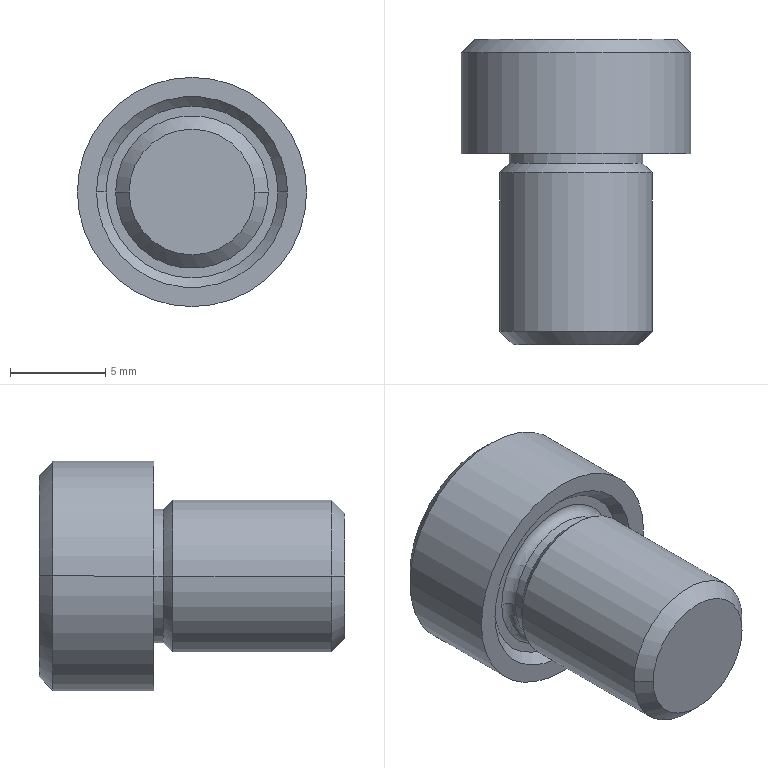Part | SolidWorks | features Revolution 1 | 1 solid | 20 faces | box 12 x 16 x 12 mm | volume 1142 mm3 | cone 8 | cylinder 6 | plane 4 | torus 2 | commonest cylinder face diameters 7 x2 8 x2 12 x2
STEP:
#1=CARTESIAN_POINT('',(-5.293,0.,0.));
#2=VERTEX_POINT('',#1);
#3=CARTESIAN_POINT('',(5.293,0.,0.));
#4=VERTEX_POINT('',#3);
#5=CARTESIAN_POINT('',(0.,0.,0.));
#6=DIRECTION('',(0.,1.,0.));
#7=DIRECTION('',(-1.,0.,0.));
#8=AXIS2_PLACEMENT_3D('',#5,#6,#7);
#9=CIRCLE('',#8,5.293);
#10=EDGE_CURVE('',#2,#4,#9,.T.);
#11=ORIENTED_EDGE('',*,*,#10,.F.);
#12=CARTESIAN_POINT('',(-6.,-0.7071,0.));
#13=VERTEX_POINT('',#12);
#14=CARTESIAN_POINT('',(-6.,-0.7071,0.));
#15=DIRECTION('',(-0.7071,-0.7071,0.));
#16=VECTOR('',#15,1000.);
#17=LINE('',#14,#16);
#18=EDGE_CURVE('',#2,#13,#17,.T.);
#19=ORIENTED_EDGE('',*,*,#18,.T.);
#20=CARTESIAN_POINT('',(6.,-0.7071,0.));
#21=VERTEX_POINT('',#20);
#22=CARTESIAN_POINT('',(0.,-0.7071,0.));
#23=DIRECTION('',(0.,1.,0.));
#24=DIRECTION('',(-1.,0.,0.));
#25=AXIS2_PLACEMENT_3D('',#22,#23,#24);
#26=CIRCLE('',#25,6.);
#27=EDGE_CURVE('',#13,#21,#26,.T.);
#28=ORIENTED_EDGE('',*,*,#27,.T.);
#29=CARTESIAN_POINT('',(6.,-0.7071,0.));
#30=DIRECTION('',(0.7071,-0.7071,0.));
#31=VECTOR('',#30,1000.);
#32=LINE('',#29,#31);
#33=EDGE_CURVE('',#4,#21,#32,.T.);
#34=ORIENTED_EDGE('',*,*,#33,.F.);
#35=EDGE_LOOP('',(#11,#19,#28,#34));
#36=FACE_OUTER_BOUND('',#35,.T.);
#37=CARTESIAN_POINT('',(0.,-0.7071,0.));
#38=DIRECTION('',(0.,-1.,0.));
#39=DIRECTION('',(1.,0.,0.));
#40=AXIS2_PLACEMENT_3D('',#37,#38,#39);
#41=CONICAL_SURFACE('',#40,6.,0.7854);
#42=ADVANCED_FACE('',(#36),#41,.T.);
#43=CARTESIAN_POINT('',(-6.,-6.,0.));
#44=VERTEX_POINT('',#43);
#45=CARTESIAN_POINT('',(6.,-6.,0.));
#46=VERTEX_POINT('',#45);
#47=CARTESIAN_POINT('',(0.,-6.,0.));
#48=DIRECTION('',(0.,1.,0.));
#49=DIRECTION('',(-1.,0.,0.));
#50=AXIS2_PLACEMENT_3D('',#47,#48,#49);
#51=CIRCLE('',#50,6.);
#52=EDGE_CURVE('',#44,#46,#51,.T.);
#53=ORIENTED_EDGE('',*,*,#52,.T.);
#54=CARTESIAN_POINT('',(6.,42.171,0.));
#55=DIRECTION('',(0.,1.,0.));
#56=VECTOR('',#55,1000.);
#57=LINE('',#54,#56);
#58=EDGE_CURVE('',#46,#21,#57,.T.);
#59=ORIENTED_EDGE('',*,*,#58,.T.);
#60=ORIENTED_EDGE('',*,*,#27,.F.);
#61=CARTESIAN_POINT('',(-6.,42.171,0.));
#62=DIRECTION('',(0.,1.,0.));
#63=VECTOR('',#62,1000.);
#64=LINE('',#61,#63);
#65=EDGE_CURVE('',#44,#13,#64,.T.);
#66=ORIENTED_EDGE('',*,*,#65,.F.);
#67=EDGE_LOOP('',(#53,#59,#60,#66));
#68=FACE_OUTER_BOUND('',#67,.T.);
#69=CARTESIAN_POINT('',(0.,42.171,0.));
#70=DIRECTION('',(0.,1.,0.));
#71=DIRECTION('',(-1.,0.,0.));
#72=AXIS2_PLACEMENT_3D('',#69,#70,#71);
#73=CYLINDRICAL_SURFACE('',#72,6.);
#74=ADVANCED_FACE('',(#68),#73,.T.);
#75=CARTESIAN_POINT('',(4.5,-5.5,0.));
#76=VERTEX_POINT('',#75);
#77=CARTESIAN_POINT('',(-4.5,-5.5,0.));
#78=VERTEX_POINT('',#77);
#79=CARTESIAN_POINT('',(0.,-5.5,0.));
#80=DIRECTION('',(0.,1.,0.));
#81=DIRECTION('',(-1.,0.,0.));
#82=AXIS2_PLACEMENT_3D('',#79,#80,#81);
#83=CIRCLE('',#82,4.5);
#84=EDGE_CURVE('',#76,#78,#83,.T.);
#85=ORIENTED_EDGE('',*,*,#84,.T.);
#86=CARTESIAN_POINT('',(-5.,-6.,0.));
#87=VERTEX_POINT('',#86);
#88=CARTESIAN_POINT('',(-4.5,-5.5,0.));
#89=DIRECTION('',(-0.7071,-0.7071,0.));
#90=VECTOR('',#89,1000.);
#91=LINE('',#88,#90);
#92=EDGE_CURVE('',#78,#87,#91,.T.);
#93=ORIENTED_EDGE('',*,*,#92,.T.);
#94=CARTESIAN_POINT('',(5.,-6.,0.));
#95=VERTEX_POINT('',#94);
#96=CARTESIAN_POINT('',(0.,-6.,0.));
#97=DIRECTION('',(0.,1.,0.));
#98=DIRECTION('',(-1.,0.,0.));
#99=AXIS2_PLACEMENT_3D('',#96,#97,#98);
#100=CIRCLE('',#99,5.);
#101=EDGE_CURVE('',#95,#87,#100,.T.);
#102=ORIENTED_EDGE('',*,*,#101,.F.);
#103=CARTESIAN_POINT('',(4.5,-5.5,0.));
#104=DIRECTION('',(0.7071,-0.7071,0.));
#105=VECTOR('',#104,1000.);
#106=LINE('',#103,#105);
#107=EDGE_CURVE('',#76,#95,#106,.T.);
#108=ORIENTED_EDGE('',*,*,#107,.F.);
#109=EDGE_LOOP('',(#85,#93,#102,#108));
#110=FACE_OUTER_BOUND('',#109,.T.);
#111=CARTESIAN_POINT('',(0.,-5.5,0.));
#112=DIRECTION('',(0.,-1.,0.));
#113=DIRECTION('',(1.,0.,0.));
#114=AXIS2_PLACEMENT_3D('',#111,#112,#113);
#115=CONICAL_SURFACE('',#114,4.5,0.7854);
#116=ADVANCED_FACE('',(#110),#115,.F.);
#117=CARTESIAN_POINT('',(4.,-5.5,0.));
#118=VERTEX_POINT('',#117);
#119=CARTESIAN_POINT('',(-4.,-5.5,0.));
#120=VERTEX_POINT('',#119);
#121=CARTESIAN_POINT('',(0.,-5.5,0.));
#122=DIRECTION('',(0.,1.,0.));
#123=DIRECTION('',(-1.,0.,0.));
#124=AXIS2_PLACEMENT_3D('',#121,#122,#123);
#125=CIRCLE('',#124,4.);
#126=EDGE_CURVE('',#118,#120,#125,.T.);
#127=ORIENTED_EDGE('',*,*,#126,.F.);
#128=CARTESIAN_POINT('',(3.5,-6.,0.));
#129=VERTEX_POINT('',#128);
#130=CARTESIAN_POINT('',(4.,-6.,0.));
#131=DIRECTION('',(0.,0.,1.));
#132=DIRECTION('',(1.,0.,0.));
#133=AXIS2_PLACEMENT_3D('',#130,#131,#132);
#134=CIRCLE('',#133,0.5);
#135=EDGE_CURVE('',#118,#129,#134,.T.);
#136=ORIENTED_EDGE('',*,*,#135,.T.);
#137=CARTESIAN_POINT('',(-3.5,-6.,0.));
#138=VERTEX_POINT('',#137);
#139=CARTESIAN_POINT('',(0.,-6.,0.));
#140=DIRECTION('',(0.,1.,0.));
#141=DIRECTION('',(-1.,0.,0.));
#142=AXIS2_PLACEMENT_3D('',#139,#140,#141);
#143=CIRCLE('',#142,3.5);
#144=EDGE_CURVE('',#129,#138,#143,.T.);
#145=ORIENTED_EDGE('',*,*,#144,.T.);
#146=CARTESIAN_POINT('',(-4.,-6.,0.));
#147=DIRECTION('',(0.,0.,-1.));
#148=DIRECTION('',(-1.,0.,0.));
#149=AXIS2_PLACEMENT_3D('',#146,#147,#148);
#150=CIRCLE('',#149,0.5);
#151=EDGE_CURVE('',#120,#138,#150,.T.);
#152=ORIENTED_EDGE('',*,*,#151,.F.);
#153=EDGE_LOOP('',(#127,#136,#145,#152));
#154=FACE_OUTER_BOUND('',#153,.T.);
#155=CARTESIAN_POINT('',(0.,-6.,0.));
#156=DIRECTION('',(0.,1.,0.));
#157=DIRECTION('',(-1.,0.,0.));
#158=AXIS2_PLACEMENT_3D('',#155,#156,#157);
#159=TOROIDAL_SURFACE('',#158,4.,0.5);
#160=ADVANCED_FACE('',(#154),#159,.F.);
#161=CARTESIAN_POINT('',(-3.5,-6.5,0.));
#162=VERTEX_POINT('',#161);
#163=CARTESIAN_POINT('',(3.5,-6.5,0.));
#164=VERTEX_POINT('',#163);
#165=CARTESIAN_POINT('',(0.,-6.5,0.));
#166=DIRECTION('',(0.,1.,0.));
#167=DIRECTION('',(-1.,0.,0.));
#168=AXIS2_PLACEMENT_3D('',#165,#166,#167);
#169=CIRCLE('',#168,3.5);
#170=EDGE_CURVE('',#162,#164,#169,.T.);
#171=ORIENTED_EDGE('',*,*,#170,.T.);
#172=CARTESIAN_POINT('',(3.5,42.171,0.));
#173=DIRECTION('',(0.,1.,0.));
#174=VECTOR('',#173,1000.);
#175=LINE('',#172,#174);
#176=EDGE_CURVE('',#164,#129,#175,.T.);
#177=ORIENTED_EDGE('',*,*,#176,.T.);
#178=CARTESIAN_POINT('',(0.,-6.,0.));
#179=DIRECTION('',(0.,1.,0.));
#180=DIRECTION('',(-1.,0.,0.));
#181=AXIS2_PLACEMENT_3D('',#178,#179,#180);
#182=CIRCLE('',#181,3.5);
#183=EDGE_CURVE('',#138,#129,#182,.T.);
#184=ORIENTED_EDGE('',*,*,#183,.F.);
#185=CARTESIAN_POINT('',(-3.5,42.171,0.));
#186=DIRECTION('',(0.,1.,0.));
#187=VECTOR('',#186,1000.);
#188=LINE('',#185,#187);
#189=EDGE_CURVE('',#162,#138,#188,.T.);
#190=ORIENTED_EDGE('',*,*,#189,.F.);
#191=EDGE_LOOP('',(#171,#177,#184,#190));
#192=FACE_OUTER_BOUND('',#191,.T.);
#193=CARTESIAN_POINT('',(0.,42.171,0.));
#194=DIRECTION('',(0.,1.,0.));
#195=DIRECTION('',(-1.,0.,0.));
#196=AXIS2_PLACEMENT_3D('',#193,#194,#195);
#197=CYLINDRICAL_SURFACE('',#196,3.5);
#198=ADVANCED_FACE('',(#192),#197,.T.);
#199=ORIENTED_EDGE('',*,*,#170,.F.);
#200=CARTESIAN_POINT('',(-4.,-7.,0.));
#201=VERTEX_POINT('',#200);
#202=CARTESIAN_POINT('',(-4.,-7.,0.));
#203=DIRECTION('',(-0.7071,-0.7071,0.));
#204=VECTOR('',#203,1000.);
#205=LINE('',#202,#204);
#206=EDGE_CURVE('',#162,#201,#205,.T.);
#207=ORIENTED_EDGE('',*,*,#206,.T.);
#208=CARTESIAN_POINT('',(4.,-7.,0.));
#209=VERTEX_POINT('',#208);
#210=CARTESIAN_POINT('',(0.,-7.,0.));
#211=DIRECTION('',(0.,1.,0.));
#212=DIRECTION('',(-1.,0.,0.));
#213=AXIS2_PLACEMENT_3D('',#210,#211,#212);
#214=CIRCLE('',#213,4.);
#215=EDGE_CURVE('',#201,#209,#214,.T.);
#216=ORIENTED_EDGE('',*,*,#215,.T.);
#217=CARTESIAN_POINT('',(4.,-7.,0.));
#218=DIRECTION('',(0.7071,-0.7071,0.));
#219=VECTOR('',#218,1000.);
#220=LINE('',#217,#219);
#221=EDGE_CURVE('',#164,#209,#220,.T.);
#222=ORIENTED_EDGE('',*,*,#221,.F.);
#223=EDGE_LOOP('',(#199,#207,#216,#222));
#224=FACE_OUTER_BOUND('',#223,.T.);
#225=CARTESIAN_POINT('',(0.,-7.,0.));
#226=DIRECTION('',(0.,-1.,0.));
#227=DIRECTION('',(1.,0.,0.));
#228=AXIS2_PLACEMENT_3D('',#225,#226,#227);
#229=CONICAL_SURFACE('',#228,4.,0.7854);
#230=ADVANCED_FACE('',(#224),#229,.T.);
#231=CARTESIAN_POINT('',(-4.,-15.293,0.));
#232=VERTEX_POINT('',#231);
#233=CARTESIAN_POINT('',(4.,-15.293,0.));
#234=VERTEX_POINT('',#233);
#235=CARTESIAN_POINT('',(0.,-15.293,0.));
#236=DIRECTION('',(0.,1.,0.));
#237=DIRECTION('',(-1.,0.,0.));
#238=AXIS2_PLACEMENT_3D('',#235,#236,#237);
#239=CIRCLE('',#238,4.);
#240=EDGE_CURVE('',#232,#234,#239,.T.);
#241=ORIENTED_EDGE('',*,*,#240,.T.);
#242=CARTESIAN_POINT('',(4.,42.171,0.));
#243=DIRECTION('',(0.,1.,0.));
#244=VECTOR('',#243,1000.);
#245=LINE('',#242,#244);
#246=EDGE_CURVE('',#234,#209,#245,.T.);
#247=ORIENTED_EDGE('',*,*,#246,.T.);
#248=ORIENTED_EDGE('',*,*,#215,.F.);
#249=CARTESIAN_POINT('',(-4.,42.171,0.));
#250=DIRECTION('',(0.,1.,0.));
#251=VECTOR('',#250,1000.);
#252=LINE('',#249,#251);
#253=EDGE_CURVE('',#232,#201,#252,.T.);
#254=ORIENTED_EDGE('',*,*,#253,.F.);
#255=EDGE_LOOP('',(#241,#247,#248,#254));
#256=FACE_OUTER_BOUND('',#255,.T.);
#257=CARTESIAN_POINT('',(0.,42.171,0.));
#258=DIRECTION('',(0.,1.,0.));
#259=DIRECTION('',(-1.,0.,0.));
#260=AXIS2_PLACEMENT_3D('',#257,#258,#259);
#261=CYLINDRICAL_SURFACE('',#260,4.);
#262=ADVANCED_FACE('',(#256),#261,.T.);
#263=CARTESIAN_POINT('',(-3.293,-16.,0.));
#264=VERTEX_POINT('',#263);
#265=CARTESIAN_POINT('',(3.293,-16.,0.));
#266=VERTEX_POINT('',#265);
#267=CARTESIAN_POINT('',(0.,-16.,0.));
#268=DIRECTION('',(0.,1.,0.));
#269=DIRECTION('',(-1.,0.,0.));
#270=AXIS2_PLACEMENT_3D('',#267,#268,#269);
#271=CIRCLE('',#270,3.293);
#272=EDGE_CURVE('',#264,#266,#271,.T.);
#273=ORIENTED_EDGE('',*,*,#272,.T.);
#274=CARTESIAN_POINT('',(3.293,-16.,0.));
#275=DIRECTION('',(0.7071,0.7071,0.));
#276=VECTOR('',#275,1000.);
#277=LINE('',#274,#276);
#278=EDGE_CURVE('',#266,#234,#277,.T.);
#279=ORIENTED_EDGE('',*,*,#278,.T.);
#280=ORIENTED_EDGE('',*,*,#240,.F.);
#281=CARTESIAN_POINT('',(-3.293,-16.,0.));
#282=DIRECTION('',(-0.7071,0.7071,0.));
#283=VECTOR('',#282,1000.);
#284=LINE('',#281,#283);
#285=EDGE_CURVE('',#264,#232,#284,.T.);
#286=ORIENTED_EDGE('',*,*,#285,.F.);
#287=EDGE_LOOP('',(#273,#279,#280,#286));
#288=FACE_OUTER_BOUND('',#287,.T.);
#289=CARTESIAN_POINT('',(0.,-16.,0.));
#290=DIRECTION('',(0.,1.,0.));
#291=DIRECTION('',(-1.,0.,0.));
#292=AXIS2_PLACEMENT_3D('',#289,#290,#291);
#293=CONICAL_SURFACE('',#292,3.293,0.7854);
#294=ADVANCED_FACE('',(#288),#293,.T.);
#295=ORIENTED_EDGE('',*,*,#272,.F.);
#296=CARTESIAN_POINT('',(0.,-16.,0.));
#297=DIRECTION('',(0.,1.,0.));
#298=DIRECTION('',(-1.,0.,0.));
#299=AXIS2_PLACEMENT_3D('',#296,#297,#298);
#300=CIRCLE('',#299,3.293);
#301=EDGE_CURVE('',#266,#264,#300,.T.);
#302=ORIENTED_EDGE('',*,*,#301,.F.);
#303=EDGE_LOOP('',(#295,#302));
#304=FACE_OUTER_BOUND('',#303,.T.);
#305=CARTESIAN_POINT('',(3.293,-16.,0.));
#306=DIRECTION('',(0.,1.,0.));
#307=DIRECTION('',(-1.,0.,0.));
#308=AXIS2_PLACEMENT_3D('',#305,#306,#307);
#309=PLANE('',#308);
#310=ADVANCED_FACE('',(#304),#309,.F.);
#311=ORIENTED_EDGE('',*,*,#278,.F.);
#312=ORIENTED_EDGE('',*,*,#301,.T.);
#313=ORIENTED_EDGE('',*,*,#285,.T.);
#314=CARTESIAN_POINT('',(0.,-15.293,0.));
#315=DIRECTION('',(0.,1.,0.));
#316=DIRECTION('',(-1.,0.,0.));
#317=AXIS2_PLACEMENT_3D('',#314,#315,#316);
#318=CIRCLE('',#317,4.);
#319=EDGE_CURVE('',#234,#232,#318,.T.);
#320=ORIENTED_EDGE('',*,*,#319,.F.);
#321=EDGE_LOOP('',(#311,#312,#313,#320));
#322=FACE_OUTER_BOUND('',#321,.T.);
#323=CARTESIAN_POINT('',(0.,-16.,0.));
#324=DIRECTION('',(0.,1.,0.));
#325=DIRECTION('',(-1.,0.,0.));
#326=AXIS2_PLACEMENT_3D('',#323,#324,#325);
#327=CONICAL_SURFACE('',#326,3.293,0.7854);
#328=ADVANCED_FACE('',(#322),#327,.T.);
#329=ORIENTED_EDGE('',*,*,#246,.F.);
#330=ORIENTED_EDGE('',*,*,#319,.T.);
#331=ORIENTED_EDGE('',*,*,#253,.T.);
#332=CARTESIAN_POINT('',(0.,-7.,0.));
#333=DIRECTION('',(0.,1.,0.));
#334=DIRECTION('',(-1.,0.,0.));
#335=AXIS2_PLACEMENT_3D('',#332,#333,#334);
#336=CIRCLE('',#335,4.);
#337=EDGE_CURVE('',#209,#201,#336,.T.);
#338=ORIENTED_EDGE('',*,*,#337,.F.);
#339=EDGE_LOOP('',(#329,#330,#331,#338));
#340=FACE_OUTER_BOUND('',#339,.T.);
#341=CARTESIAN_POINT('',(0.,42.171,0.));
#342=DIRECTION('',(0.,1.,0.));
#343=DIRECTION('',(-1.,0.,0.));
#344=AXIS2_PLACEMENT_3D('',#341,#342,#343);
#345=CYLINDRICAL_SURFACE('',#344,4.);
#346=ADVANCED_FACE('',(#340),#345,.T.);
#347=ORIENTED_EDGE('',*,*,#206,.F.);
#348=CARTESIAN_POINT('',(0.,-6.5,0.));
#349=DIRECTION('',(0.,1.,0.));
#350=DIRECTION('',(-1.,0.,0.));
#351=AXIS2_PLACEMENT_3D('',#348,#349,#350);
#352=CIRCLE('',#351,3.5);
#353=EDGE_CURVE('',#164,#162,#352,.T.);
#354=ORIENTED_EDGE('',*,*,#353,.F.);
#355=ORIENTED_EDGE('',*,*,#221,.T.);
#356=ORIENTED_EDGE('',*,*,#337,.T.);
#357=EDGE_LOOP('',(#347,#354,#355,#356));
#358=FACE_OUTER_BOUND('',#357,.T.);
#359=CARTESIAN_POINT('',(0.,-7.,0.));
#360=DIRECTION('',(0.,-1.,0.));
#361=DIRECTION('',(1.,0.,0.));
#362=AXIS2_PLACEMENT_3D('',#359,#360,#361);
#363=CONICAL_SURFACE('',#362,4.,0.7854);
#364=ADVANCED_FACE('',(#358),#363,.T.);
#365=ORIENTED_EDGE('',*,*,#176,.F.);
#366=ORIENTED_EDGE('',*,*,#353,.T.);
#367=ORIENTED_EDGE('',*,*,#189,.T.);
#368=ORIENTED_EDGE('',*,*,#144,.F.);
#369=EDGE_LOOP('',(#365,#366,#367,#368));
#370=FACE_OUTER_BOUND('',#369,.T.);
#371=CARTESIAN_POINT('',(0.,42.171,0.));
#372=DIRECTION('',(0.,1.,0.));
#373=DIRECTION('',(-1.,0.,0.));
#374=AXIS2_PLACEMENT_3D('',#371,#372,#373);
#375=CYLINDRICAL_SURFACE('',#374,3.5);
#376=ADVANCED_FACE('',(#370),#375,.T.);
#377=ORIENTED_EDGE('',*,*,#135,.F.);
#378=CARTESIAN_POINT('',(0.,-5.5,0.));
#379=DIRECTION('',(0.,1.,0.));
#380=DIRECTION('',(-1.,0.,0.));
#381=AXIS2_PLACEMENT_3D('',#378,#379,#380);
#382=CIRCLE('',#381,4.);
#383=EDGE_CURVE('',#120,#118,#382,.T.);
#384=ORIENTED_EDGE('',*,*,#383,.F.);
#385=ORIENTED_EDGE('',*,*,#151,.T.);
#386=ORIENTED_EDGE('',*,*,#183,.T.);
#387=EDGE_LOOP('',(#377,#384,#385,#386));
#388=FACE_OUTER_BOUND('',#387,.T.);
#389=CARTESIAN_POINT('',(0.,-6.,0.));
#390=DIRECTION('',(0.,1.,0.));
#391=DIRECTION('',(-1.,0.,0.));
#392=AXIS2_PLACEMENT_3D('',#389,#390,#391);
#393=TOROIDAL_SURFACE('',#392,4.,0.5);
#394=ADVANCED_FACE('',(#388),#393,.F.);
#395=ORIENTED_EDGE('',*,*,#84,.F.);
#396=CARTESIAN_POINT('',(0.,-5.5,0.));
#397=DIRECTION('',(0.,1.,0.));
#398=DIRECTION('',(-1.,0.,0.));
#399=AXIS2_PLACEMENT_3D('',#396,#397,#398);
#400=CIRCLE('',#399,4.5);
#401=EDGE_CURVE('',#78,#76,#400,.T.);
#402=ORIENTED_EDGE('',*,*,#401,.F.);
#403=EDGE_LOOP('',(#395,#402));
#404=FACE_OUTER_BOUND('',#403,.T.);
#405=ORIENTED_EDGE('',*,*,#383,.T.);
#406=ORIENTED_EDGE('',*,*,#126,.T.);
#407=EDGE_LOOP('',(#405,#406));
#408=FACE_BOUND('',#407,.T.);
#409=CARTESIAN_POINT('',(4.5,-5.5,0.));
#410=DIRECTION('',(0.,1.,0.));
#411=DIRECTION('',(-1.,0.,0.));
#412=AXIS2_PLACEMENT_3D('',#409,#410,#411);
#413=PLANE('',#412);
#414=ADVANCED_FACE('',(#404,#408),#413,.F.);
#415=ORIENTED_EDGE('',*,*,#92,.F.);
#416=ORIENTED_EDGE('',*,*,#401,.T.);
#417=ORIENTED_EDGE('',*,*,#107,.T.);
#418=CARTESIAN_POINT('',(0.,-6.,0.));
#419=DIRECTION('',(0.,1.,0.));
#420=DIRECTION('',(-1.,0.,0.));
#421=AXIS2_PLACEMENT_3D('',#418,#419,#420);
#422=CIRCLE('',#421,5.);
#423=EDGE_CURVE('',#87,#95,#422,.T.);
#424=ORIENTED_EDGE('',*,*,#423,.F.);
#425=EDGE_LOOP('',(#415,#416,#417,#424));
#426=FACE_OUTER_BOUND('',#425,.T.);
#427=CARTESIAN_POINT('',(0.,-5.5,0.));
#428=DIRECTION('',(0.,-1.,0.));
#429=DIRECTION('',(1.,0.,0.));
#430=AXIS2_PLACEMENT_3D('',#427,#428,#429);
#431=CONICAL_SURFACE('',#430,4.5,0.7854);
#432=ADVANCED_FACE('',(#426),#431,.F.);
#433=ORIENTED_EDGE('',*,*,#52,.F.);
#434=CARTESIAN_POINT('',(0.,-6.,0.));
#435=DIRECTION('',(0.,1.,0.));
#436=DIRECTION('',(-1.,0.,0.));
#437=AXIS2_PLACEMENT_3D('',#434,#435,#436);
#438=CIRCLE('',#437,6.);
#439=EDGE_CURVE('',#46,#44,#438,.T.);
#440=ORIENTED_EDGE('',*,*,#439,.F.);
#441=EDGE_LOOP('',(#433,#440));
#442=FACE_OUTER_BOUND('',#441,.T.);
#443=ORIENTED_EDGE('',*,*,#101,.T.);
#444=ORIENTED_EDGE('',*,*,#423,.T.);
#445=EDGE_LOOP('',(#443,#444));
#446=FACE_BOUND('',#445,.T.);
#447=CARTESIAN_POINT('',(6.,-6.,0.));
#448=DIRECTION('',(0.,1.,0.));
#449=DIRECTION('',(-1.,0.,0.));
#450=AXIS2_PLACEMENT_3D('',#447,#448,#449);
#451=PLANE('',#450);
#452=ADVANCED_FACE('',(#442,#446),#451,.F.);
#453=ORIENTED_EDGE('',*,*,#58,.F.);
#454=ORIENTED_EDGE('',*,*,#439,.T.);
#455=ORIENTED_EDGE('',*,*,#65,.T.);
#456=CARTESIAN_POINT('',(0.,-0.7071,0.));
#457=DIRECTION('',(0.,1.,0.));
#458=DIRECTION('',(-1.,0.,0.));
#459=AXIS2_PLACEMENT_3D('',#456,#457,#458);
#460=CIRCLE('',#459,6.);
#461=EDGE_CURVE('',#21,#13,#460,.T.);
#462=ORIENTED_EDGE('',*,*,#461,.F.);
#463=EDGE_LOOP('',(#453,#454,#455,#462));
#464=FACE_OUTER_BOUND('',#463,.T.);
#465=CARTESIAN_POINT('',(0.,42.171,0.));
#466=DIRECTION('',(0.,1.,0.));
#467=DIRECTION('',(-1.,0.,0.));
#468=AXIS2_PLACEMENT_3D('',#465,#466,#467);
#469=CYLINDRICAL_SURFACE('',#468,6.);
#470=ADVANCED_FACE('',(#464),#469,.T.);
#471=ORIENTED_EDGE('',*,*,#18,.F.);
#472=CARTESIAN_POINT('',(0.,0.,0.));
#473=DIRECTION('',(0.,1.,0.));
#474=DIRECTION('',(-1.,0.,0.));
#475=AXIS2_PLACEMENT_3D('',#472,#473,#474);
#476=CIRCLE('',#475,5.293);
#477=EDGE_CURVE('',#4,#2,#476,.T.);
#478=ORIENTED_EDGE('',*,*,#477,.F.);
#479=ORIENTED_EDGE('',*,*,#33,.T.);
#480=ORIENTED_EDGE('',*,*,#461,.T.);
#481=EDGE_LOOP('',(#471,#478,#479,#480));
#482=FACE_OUTER_BOUND('',#481,.T.);
#483=CARTESIAN_POINT('',(0.,-0.7071,0.));
#484=DIRECTION('',(0.,-1.,0.));
#485=DIRECTION('',(1.,0.,0.));
#486=AXIS2_PLACEMENT_3D('',#483,#484,#485);
#487=CONICAL_SURFACE('',#486,6.,0.7854);
#488=ADVANCED_FACE('',(#482),#487,.T.);
#489=ORIENTED_EDGE('',*,*,#477,.T.);
#490=ORIENTED_EDGE('',*,*,#10,.T.);
#491=EDGE_LOOP('',(#489,#490));
#492=FACE_OUTER_BOUND('',#491,.T.);
#493=CARTESIAN_POINT('',(0.,0.,0.));
#494=DIRECTION('',(0.,-1.,0.));
#495=DIRECTION('',(1.,0.,0.));
#496=AXIS2_PLACEMENT_3D('',#493,#494,#495);
#497=PLANE('',#496);
#498=ADVANCED_FACE('',(#492),#497,.F.);
#499=CLOSED_SHELL('',(#42,#74,#116,#160,#198,#230,#262,#294,#310,#328,#346,#364,#376,#394,#414,#432,#452,#470,#488,#498));
#500=MANIFOLD_SOLID_BREP('',#499);
#501=CARTESIAN_POINT('',(0.,0.,0.));
#502=DIRECTION('',(0.,0.,1.));
#503=DIRECTION('',(1.,0.,0.));
#504=AXIS2_PLACEMENT_3D('',#501,#502,#503);
#505=(LENGTH_UNIT()NAMED_UNIT(*)SI_UNIT(.MILLI.,.METRE.));
#506=UNCERTAINTY_MEASURE_WITH_UNIT(LENGTH_MEASURE(0.00001),#505,'','');
#507=(NAMED_UNIT(*)PLANE_ANGLE_UNIT()SI_UNIT($,.RADIAN.));
#508=(NAMED_UNIT(*)SI_UNIT($,.STERADIAN.)SOLID_ANGLE_UNIT());
#509=(GEOMETRIC_REPRESENTATION_CONTEXT(3)GLOBAL_UNCERTAINTY_ASSIGNED_CONTEXT((#506))GLOBAL_UNIT_ASSIGNED_CONTEXT((#505,#507,#508))REPRESENTATION_CONTEXT('',''));
#510=ADVANCED_BREP_SHAPE_REPRESENTATION('',(#500,#504),#509);